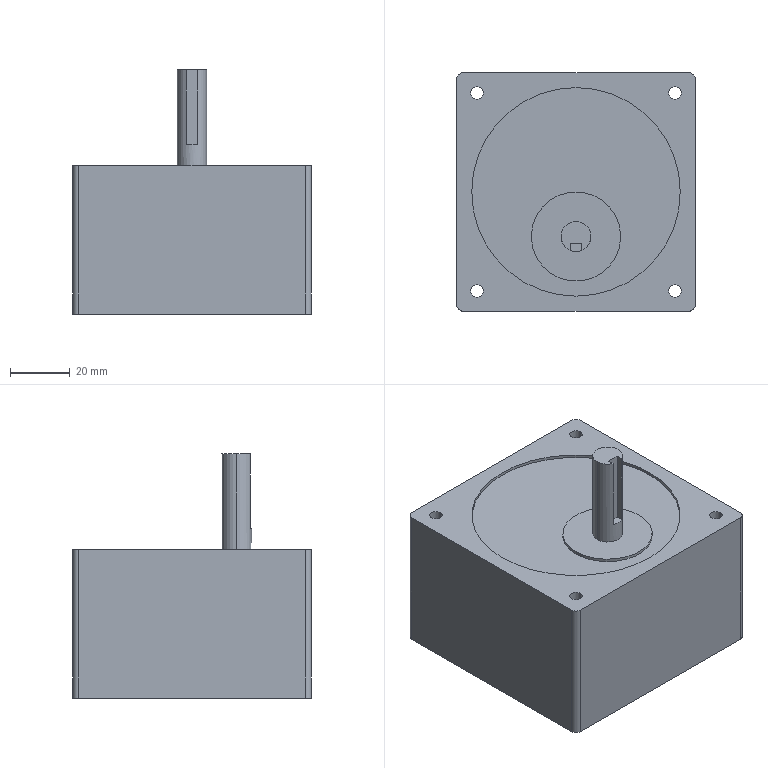Part | SolidWorks | features ICE 5, 3DProfileFeature 1, Extrusion 1, Fillet 1, HoleWzd 1 | 1 solid | 34 faces | box 80 x 80 x 82 mm | volume 314622 mm3 | cylinder 20 | plane 14 | commonest cylinder face diameters 4.2 x8 4 x4 10 x4 30 x2 70 x2
STEP:
#1=CARTESIAN_POINT('',(45.,25.,82.));
#2=VERTEX_POINT('',#1);
#3=CARTESIAN_POINT('',(35.,25.,82.));
#4=VERTEX_POINT('',#3);
#5=CARTESIAN_POINT('',(40.,25.,82.));
#6=DIRECTION('',(0.,0.,1.));
#7=DIRECTION('',(1.,0.,0.));
#8=AXIS2_PLACEMENT_3D('',#5,#6,#7);
#9=CIRCLE('',#8,5.);
#10=EDGE_CURVE('',#2,#4,#9,.T.);
#11=ORIENTED_EDGE('',*,*,#10,.F.);
#12=CARTESIAN_POINT('',(45.,25.,50.));
#13=VERTEX_POINT('',#12);
#14=CARTESIAN_POINT('',(45.,25.,82.));
#15=DIRECTION('',(0.,0.,-1.));
#16=VECTOR('',#15,1000.);
#17=LINE('',#14,#16);
#18=EDGE_CURVE('',#2,#13,#17,.T.);
#19=ORIENTED_EDGE('',*,*,#18,.T.);
#20=CARTESIAN_POINT('',(35.,25.,50.));
#21=VERTEX_POINT('',#20);
#22=CARTESIAN_POINT('',(40.,25.,50.));
#23=DIRECTION('',(0.,0.,1.));
#24=DIRECTION('',(1.,0.,0.));
#25=AXIS2_PLACEMENT_3D('',#22,#23,#24);
#26=CIRCLE('',#25,5.);
#27=EDGE_CURVE('',#13,#21,#26,.T.);
#28=ORIENTED_EDGE('',*,*,#27,.T.);
#29=CARTESIAN_POINT('',(35.,25.,82.));
#30=DIRECTION('',(0.,0.,-1.));
#31=VECTOR('',#30,1000.);
#32=LINE('',#29,#31);
#33=EDGE_CURVE('',#4,#21,#32,.T.);
#34=ORIENTED_EDGE('',*,*,#33,.F.);
#35=EDGE_LOOP('',(#11,#19,#28,#34));
#36=FACE_OUTER_BOUND('',#35,.T.);
#37=CARTESIAN_POINT('',(40.,25.,82.));
#38=DIRECTION('',(0.,0.,-1.));
#39=DIRECTION('',(-1.,0.,0.));
#40=AXIS2_PLACEMENT_3D('',#37,#38,#39);
#41=CYLINDRICAL_SURFACE('',#40,5.);
#42=ADVANCED_FACE('',(#36),#41,.T.);
#43=CARTESIAN_POINT('',(55.,25.,50.));
#44=VERTEX_POINT('',#43);
#45=CARTESIAN_POINT('',(25.,25.,50.));
#46=VERTEX_POINT('',#45);
#47=CARTESIAN_POINT('',(40.,25.,50.));
#48=DIRECTION('',(0.,0.,1.));
#49=DIRECTION('',(1.,0.,0.));
#50=AXIS2_PLACEMENT_3D('',#47,#48,#49);
#51=CIRCLE('',#50,15.);
#52=EDGE_CURVE('',#44,#46,#51,.T.);
#53=ORIENTED_EDGE('',*,*,#52,.F.);
#54=CARTESIAN_POINT('',(55.,25.,49.));
#55=VERTEX_POINT('',#54);
#56=CARTESIAN_POINT('',(55.,25.,50.));
#57=DIRECTION('',(0.,0.,-1.));
#58=VECTOR('',#57,1000.);
#59=LINE('',#56,#58);
#60=EDGE_CURVE('',#44,#55,#59,.T.);
#61=ORIENTED_EDGE('',*,*,#60,.T.);
#62=CARTESIAN_POINT('',(25.,25.,49.));
#63=VERTEX_POINT('',#62);
#64=CARTESIAN_POINT('',(40.,25.,49.));
#65=DIRECTION('',(0.,0.,1.));
#66=DIRECTION('',(1.,0.,0.));
#67=AXIS2_PLACEMENT_3D('',#64,#65,#66);
#68=CIRCLE('',#67,15.);
#69=EDGE_CURVE('',#55,#63,#68,.T.);
#70=ORIENTED_EDGE('',*,*,#69,.T.);
#71=CARTESIAN_POINT('',(25.,25.,50.));
#72=DIRECTION('',(0.,0.,-1.));
#73=VECTOR('',#72,1000.);
#74=LINE('',#71,#73);
#75=EDGE_CURVE('',#46,#63,#74,.T.);
#76=ORIENTED_EDGE('',*,*,#75,.F.);
#77=EDGE_LOOP('',(#53,#61,#70,#76));
#78=FACE_OUTER_BOUND('',#77,.T.);
#79=CARTESIAN_POINT('',(40.,25.,50.));
#80=DIRECTION('',(0.,0.,-1.));
#81=DIRECTION('',(-1.,0.,0.));
#82=AXIS2_PLACEMENT_3D('',#79,#80,#81);
#83=CYLINDRICAL_SURFACE('',#82,15.);
#84=ADVANCED_FACE('',(#78),#83,.T.);
#85=CARTESIAN_POINT('',(45.,40.,20.));
#86=VERTEX_POINT('',#85);
#87=CARTESIAN_POINT('',(35.,40.,20.));
#88=VERTEX_POINT('',#87);
#89=CARTESIAN_POINT('',(40.,40.,20.));
#90=DIRECTION('',(0.,0.,-1.));
#91=DIRECTION('',(-1.,0.,0.));
#92=AXIS2_PLACEMENT_3D('',#89,#90,#91);
#93=CIRCLE('',#92,5.);
#94=EDGE_CURVE('',#86,#88,#93,.T.);
#95=ORIENTED_EDGE('',*,*,#94,.F.);
#96=CARTESIAN_POINT('',(45.,40.,0.));
#97=VERTEX_POINT('',#96);
#98=CARTESIAN_POINT('',(45.,40.,20.));
#99=DIRECTION('',(0.,0.,-1.));
#100=VECTOR('',#99,1000.);
#101=LINE('',#98,#100);
#102=EDGE_CURVE('',#86,#97,#101,.T.);
#103=ORIENTED_EDGE('',*,*,#102,.T.);
#104=CARTESIAN_POINT('',(35.,40.,0.));
#105=VERTEX_POINT('',#104);
#106=CARTESIAN_POINT('',(40.,40.,0.));
#107=DIRECTION('',(0.,0.,-1.));
#108=DIRECTION('',(-1.,0.,0.));
#109=AXIS2_PLACEMENT_3D('',#106,#107,#108);
#110=CIRCLE('',#109,5.);
#111=EDGE_CURVE('',#97,#105,#110,.T.);
#112=ORIENTED_EDGE('',*,*,#111,.T.);
#113=CARTESIAN_POINT('',(35.,40.,20.));
#114=DIRECTION('',(0.,0.,-1.));
#115=VECTOR('',#114,1000.);
#116=LINE('',#113,#115);
#117=EDGE_CURVE('',#88,#105,#116,.T.);
#118=ORIENTED_EDGE('',*,*,#117,.F.);
#119=EDGE_LOOP('',(#95,#103,#112,#118));
#120=FACE_OUTER_BOUND('',#119,.T.);
#121=CARTESIAN_POINT('',(40.,40.,20.));
#122=DIRECTION('',(0.,0.,-1.));
#123=DIRECTION('',(-1.,0.,0.));
#124=AXIS2_PLACEMENT_3D('',#121,#122,#123);
#125=CYLINDRICAL_SURFACE('',#124,5.);
#126=ADVANCED_FACE('',(#120),#125,.F.);
#127=CARTESIAN_POINT('',(75.334,73.234,50.));
#128=VERTEX_POINT('',#127);
#129=CARTESIAN_POINT('',(71.134,73.234,50.));
#130=VERTEX_POINT('',#129);
#131=CARTESIAN_POINT('',(73.234,73.234,50.));
#132=DIRECTION('',(0.,0.,-1.));
#133=DIRECTION('',(-1.,0.,0.));
#134=AXIS2_PLACEMENT_3D('',#131,#132,#133);
#135=CIRCLE('',#134,2.1);
#136=EDGE_CURVE('',#128,#130,#135,.T.);
#137=ORIENTED_EDGE('',*,*,#136,.F.);
#138=CARTESIAN_POINT('',(75.334,73.234,0.));
#139=VERTEX_POINT('',#138);
#140=CARTESIAN_POINT('',(75.334,73.234,0.));
#141=DIRECTION('',(0.,0.,-1.));
#142=VECTOR('',#141,1000.);
#143=LINE('',#140,#142);
#144=EDGE_CURVE('',#128,#139,#143,.T.);
#145=ORIENTED_EDGE('',*,*,#144,.T.);
#146=CARTESIAN_POINT('',(71.134,73.234,0.));
#147=VERTEX_POINT('',#146);
#148=CARTESIAN_POINT('',(73.234,73.234,0.));
#149=DIRECTION('',(0.,0.,-1.));
#150=DIRECTION('',(-1.,0.,0.));
#151=AXIS2_PLACEMENT_3D('',#148,#149,#150);
#152=CIRCLE('',#151,2.1);
#153=EDGE_CURVE('',#139,#147,#152,.T.);
#154=ORIENTED_EDGE('',*,*,#153,.T.);
#155=CARTESIAN_POINT('',(71.134,73.234,0.));
#156=DIRECTION('',(0.,0.,-1.));
#157=VECTOR('',#156,1000.);
#158=LINE('',#155,#157);
#159=EDGE_CURVE('',#130,#147,#158,.T.);
#160=ORIENTED_EDGE('',*,*,#159,.F.);
#161=EDGE_LOOP('',(#137,#145,#154,#160));
#162=FACE_OUTER_BOUND('',#161,.T.);
#163=CARTESIAN_POINT('',(73.234,73.234,0.));
#164=DIRECTION('',(0.,0.,-1.));
#165=DIRECTION('',(-1.,0.,0.));
#166=AXIS2_PLACEMENT_3D('',#163,#164,#165);
#167=CYLINDRICAL_SURFACE('',#166,2.1);
#168=ADVANCED_FACE('',(#162),#167,.F.);
#169=CARTESIAN_POINT('',(8.866,73.234,50.));
#170=VERTEX_POINT('',#169);
#171=CARTESIAN_POINT('',(4.666,73.234,50.));
#172=VERTEX_POINT('',#171);
#173=CARTESIAN_POINT('',(6.766,73.234,50.));
#174=DIRECTION('',(0.,0.,-1.));
#175=DIRECTION('',(-1.,0.,0.));
#176=AXIS2_PLACEMENT_3D('',#173,#174,#175);
#177=CIRCLE('',#176,2.1);
#178=EDGE_CURVE('',#170,#172,#177,.T.);
#179=ORIENTED_EDGE('',*,*,#178,.F.);
#180=CARTESIAN_POINT('',(8.866,73.234,0.));
#181=VERTEX_POINT('',#180);
#182=CARTESIAN_POINT('',(8.866,73.234,0.));
#183=DIRECTION('',(0.,0.,-1.));
#184=VECTOR('',#183,1000.);
#185=LINE('',#182,#184);
#186=EDGE_CURVE('',#170,#181,#185,.T.);
#187=ORIENTED_EDGE('',*,*,#186,.T.);
#188=CARTESIAN_POINT('',(4.666,73.234,0.));
#189=VERTEX_POINT('',#188);
#190=CARTESIAN_POINT('',(6.766,73.234,0.));
#191=DIRECTION('',(0.,0.,-1.));
#192=DIRECTION('',(-1.,0.,0.));
#193=AXIS2_PLACEMENT_3D('',#190,#191,#192);
#194=CIRCLE('',#193,2.1);
#195=EDGE_CURVE('',#181,#189,#194,.T.);
#196=ORIENTED_EDGE('',*,*,#195,.T.);
#197=CARTESIAN_POINT('',(4.666,73.234,0.));
#198=DIRECTION('',(0.,0.,-1.));
#199=VECTOR('',#198,1000.);
#200=LINE('',#197,#199);
#201=EDGE_CURVE('',#172,#189,#200,.T.);
#202=ORIENTED_EDGE('',*,*,#201,.F.);
#203=EDGE_LOOP('',(#179,#187,#196,#202));
#204=FACE_OUTER_BOUND('',#203,.T.);
#205=CARTESIAN_POINT('',(6.766,73.234,0.));
#206=DIRECTION('',(0.,0.,-1.));
#207=DIRECTION('',(-1.,0.,0.));
#208=AXIS2_PLACEMENT_3D('',#205,#206,#207);
#209=CYLINDRICAL_SURFACE('',#208,2.1);
#210=ADVANCED_FACE('',(#204),#209,.F.);
#211=CARTESIAN_POINT('',(8.866,6.766,50.));
#212=VERTEX_POINT('',#211);
#213=CARTESIAN_POINT('',(4.666,6.766,50.));
#214=VERTEX_POINT('',#213);
#215=CARTESIAN_POINT('',(6.766,6.766,50.));
#216=DIRECTION('',(0.,0.,-1.));
#217=DIRECTION('',(-1.,0.,0.));
#218=AXIS2_PLACEMENT_3D('',#215,#216,#217);
#219=CIRCLE('',#218,2.1);
#220=EDGE_CURVE('',#212,#214,#219,.T.);
#221=ORIENTED_EDGE('',*,*,#220,.F.);
#222=CARTESIAN_POINT('',(8.866,6.766,0.));
#223=VERTEX_POINT('',#222);
#224=CARTESIAN_POINT('',(8.866,6.766,0.));
#225=DIRECTION('',(0.,0.,-1.));
#226=VECTOR('',#225,1000.);
#227=LINE('',#224,#226);
#228=EDGE_CURVE('',#212,#223,#227,.T.);
#229=ORIENTED_EDGE('',*,*,#228,.T.);
#230=CARTESIAN_POINT('',(4.666,6.766,0.));
#231=VERTEX_POINT('',#230);
#232=CARTESIAN_POINT('',(6.766,6.766,0.));
#233=DIRECTION('',(0.,0.,-1.));
#234=DIRECTION('',(-1.,0.,0.));
#235=AXIS2_PLACEMENT_3D('',#232,#233,#234);
#236=CIRCLE('',#235,2.1);
#237=EDGE_CURVE('',#223,#231,#236,.T.);
#238=ORIENTED_EDGE('',*,*,#237,.T.);
#239=CARTESIAN_POINT('',(4.666,6.766,0.));
#240=DIRECTION('',(0.,0.,-1.));
#241=VECTOR('',#240,1000.);
#242=LINE('',#239,#241);
#243=EDGE_CURVE('',#214,#231,#242,.T.);
#244=ORIENTED_EDGE('',*,*,#243,.F.);
#245=EDGE_LOOP('',(#221,#229,#238,#244));
#246=FACE_OUTER_BOUND('',#245,.T.);
#247=CARTESIAN_POINT('',(6.766,6.766,0.));
#248=DIRECTION('',(0.,0.,-1.));
#249=DIRECTION('',(-1.,0.,0.));
#250=AXIS2_PLACEMENT_3D('',#247,#248,#249);
#251=CYLINDRICAL_SURFACE('',#250,2.1);
#252=ADVANCED_FACE('',(#246),#251,.F.);
#253=CARTESIAN_POINT('',(75.334,6.766,50.));
#254=VERTEX_POINT('',#253);
#255=CARTESIAN_POINT('',(71.134,6.766,50.));
#256=VERTEX_POINT('',#255);
#257=CARTESIAN_POINT('',(73.234,6.766,50.));
#258=DIRECTION('',(0.,0.,-1.));
#259=DIRECTION('',(-1.,0.,0.));
#260=AXIS2_PLACEMENT_3D('',#257,#258,#259);
#261=CIRCLE('',#260,2.1);
#262=EDGE_CURVE('',#254,#256,#261,.T.);
#263=ORIENTED_EDGE('',*,*,#262,.F.);
#264=CARTESIAN_POINT('',(75.334,6.766,0.));
#265=VERTEX_POINT('',#264);
#266=CARTESIAN_POINT('',(75.334,6.766,0.));
#267=DIRECTION('',(0.,0.,-1.));
#268=VECTOR('',#267,1000.);
#269=LINE('',#266,#268);
#270=EDGE_CURVE('',#254,#265,#269,.T.);
#271=ORIENTED_EDGE('',*,*,#270,.T.);
#272=CARTESIAN_POINT('',(71.134,6.766,0.));
#273=VERTEX_POINT('',#272);
#274=CARTESIAN_POINT('',(73.234,6.766,0.));
#275=DIRECTION('',(0.,0.,-1.));
#276=DIRECTION('',(-1.,0.,0.));
#277=AXIS2_PLACEMENT_3D('',#274,#275,#276);
#278=CIRCLE('',#277,2.1);
#279=EDGE_CURVE('',#265,#273,#278,.T.);
#280=ORIENTED_EDGE('',*,*,#279,.T.);
#281=CARTESIAN_POINT('',(71.134,6.766,0.));
#282=DIRECTION('',(0.,0.,-1.));
#283=VECTOR('',#282,1000.);
#284=LINE('',#281,#283);
#285=EDGE_CURVE('',#256,#273,#284,.T.);
#286=ORIENTED_EDGE('',*,*,#285,.F.);
#287=EDGE_LOOP('',(#263,#271,#280,#286));
#288=FACE_OUTER_BOUND('',#287,.T.);
#289=CARTESIAN_POINT('',(73.234,6.766,0.));
#290=DIRECTION('',(0.,0.,-1.));
#291=DIRECTION('',(-1.,0.,0.));
#292=AXIS2_PLACEMENT_3D('',#289,#290,#291);
#293=CYLINDRICAL_SURFACE('',#292,2.1);
#294=ADVANCED_FACE('',(#288),#293,.F.);
#295=CARTESIAN_POINT('',(5.,40.,49.));
#296=VERTEX_POINT('',#295);
#297=CARTESIAN_POINT('',(75.,40.,49.));
#298=VERTEX_POINT('',#297);
#299=CARTESIAN_POINT('',(40.,40.,49.));
#300=DIRECTION('',(0.,0.,1.));
#301=DIRECTION('',(1.,0.,0.));
#302=AXIS2_PLACEMENT_3D('',#299,#300,#301);
#303=CIRCLE('',#302,35.);
#304=EDGE_CURVE('',#296,#298,#303,.T.);
#305=ORIENTED_EDGE('',*,*,#304,.F.);
#306=CARTESIAN_POINT('',(5.,40.,50.));
#307=VERTEX_POINT('',#306);
#308=CARTESIAN_POINT('',(5.,40.,49.));
#309=DIRECTION('',(0.,0.,1.));
#310=VECTOR('',#309,1000.);
#311=LINE('',#308,#310);
#312=EDGE_CURVE('',#296,#307,#311,.T.);
#313=ORIENTED_EDGE('',*,*,#312,.T.);
#314=CARTESIAN_POINT('',(75.,40.,50.));
#315=VERTEX_POINT('',#314);
#316=CARTESIAN_POINT('',(40.,40.,50.));
#317=DIRECTION('',(0.,0.,1.));
#318=DIRECTION('',(1.,0.,0.));
#319=AXIS2_PLACEMENT_3D('',#316,#317,#318);
#320=CIRCLE('',#319,35.);
#321=EDGE_CURVE('',#307,#315,#320,.T.);
#322=ORIENTED_EDGE('',*,*,#321,.T.);
#323=CARTESIAN_POINT('',(75.,40.,49.));
#324=DIRECTION('',(0.,0.,1.));
#325=VECTOR('',#324,1000.);
#326=LINE('',#323,#325);
#327=EDGE_CURVE('',#298,#315,#326,.T.);
#328=ORIENTED_EDGE('',*,*,#327,.F.);
#329=EDGE_LOOP('',(#305,#313,#322,#328));
#330=FACE_OUTER_BOUND('',#329,.T.);
#331=CARTESIAN_POINT('',(40.,40.,49.));
#332=DIRECTION('',(0.,0.,1.));
#333=DIRECTION('',(1.,0.,0.));
#334=AXIS2_PLACEMENT_3D('',#331,#332,#333);
#335=CYLINDRICAL_SURFACE('',#334,35.);
#336=ADVANCED_FACE('',(#330),#335,.F.);
#337=CARTESIAN_POINT('',(40.,25.,50.));
#338=DIRECTION('',(0.,0.,1.));
#339=DIRECTION('',(1.,0.,0.));
#340=AXIS2_PLACEMENT_3D('',#337,#338,#339);
#341=CIRCLE('',#340,15.);
#342=EDGE_CURVE('',#46,#44,#341,.T.);
#343=ORIENTED_EDGE('',*,*,#342,.T.);
#344=ORIENTED_EDGE('',*,*,#52,.T.);
#345=EDGE_LOOP('',(#343,#344));
#346=FACE_OUTER_BOUND('',#345,.T.);
#347=CARTESIAN_POINT('',(40.,25.,50.));
#348=DIRECTION('',(0.,0.,1.));
#349=DIRECTION('',(1.,0.,0.));
#350=AXIS2_PLACEMENT_3D('',#347,#348,#349);
#351=CIRCLE('',#350,5.);
#352=EDGE_CURVE('',#21,#13,#351,.T.);
#353=ORIENTED_EDGE('',*,*,#352,.F.);
#354=ORIENTED_EDGE('',*,*,#27,.F.);
#355=EDGE_LOOP('',(#353,#354));
#356=FACE_BOUND('',#355,.T.);
#357=CARTESIAN_POINT('',(40.,25.,50.));
#358=DIRECTION('',(0.,0.,1.));
#359=DIRECTION('',(1.,0.,0.));
#360=AXIS2_PLACEMENT_3D('',#357,#358,#359);
#361=PLANE('',#360);
#362=ADVANCED_FACE('',(#346,#356),#361,.T.);
#363=CARTESIAN_POINT('',(40.,40.,49.));
#364=DIRECTION('',(0.,0.,1.));
#365=DIRECTION('',(1.,0.,0.));
#366=AXIS2_PLACEMENT_3D('',#363,#364,#365);
#367=CIRCLE('',#366,35.);
#368=EDGE_CURVE('',#298,#296,#367,.T.);
#369=ORIENTED_EDGE('',*,*,#368,.T.);
#370=ORIENTED_EDGE('',*,*,#304,.T.);
#371=EDGE_LOOP('',(#369,#370));
#372=FACE_OUTER_BOUND('',#371,.T.);
#373=CARTESIAN_POINT('',(40.,25.,49.));
#374=DIRECTION('',(0.,0.,1.));
#375=DIRECTION('',(1.,0.,0.));
#376=AXIS2_PLACEMENT_3D('',#373,#374,#375);
#377=CIRCLE('',#376,15.);
#378=EDGE_CURVE('',#63,#55,#377,.T.);
#379=ORIENTED_EDGE('',*,*,#378,.F.);
#380=ORIENTED_EDGE('',*,*,#69,.F.);
#381=EDGE_LOOP('',(#379,#380));
#382=FACE_BOUND('',#381,.T.);
#383=CARTESIAN_POINT('',(40.,40.,49.));
#384=DIRECTION('',(0.,0.,1.));
#385=DIRECTION('',(1.,0.,0.));
#386=AXIS2_PLACEMENT_3D('',#383,#384,#385);
#387=PLANE('',#386);
#388=ADVANCED_FACE('',(#372,#382),#387,.T.);
#389=CARTESIAN_POINT('',(0.,78.,50.));
#390=VERTEX_POINT('',#389);
#391=CARTESIAN_POINT('',(0.,2.,50.));
#392=VERTEX_POINT('',#391);
#393=CARTESIAN_POINT('',(0.,0.,50.));
#394=DIRECTION('',(0.,-1.,0.));
#395=VECTOR('',#394,1000.);
#396=LINE('',#393,#395);
#397=EDGE_CURVE('',#390,#392,#396,.T.);
#398=ORIENTED_EDGE('',*,*,#397,.F.);
#399=CARTESIAN_POINT('',(0.,78.,0.));
#400=VERTEX_POINT('',#399);
#401=CARTESIAN_POINT('',(0.,78.,50.));
#402=DIRECTION('',(0.,0.,-1.));
#403=VECTOR('',#402,1000.);
#404=LINE('',#401,#403);
#405=EDGE_CURVE('',#390,#400,#404,.T.);
#406=ORIENTED_EDGE('',*,*,#405,.T.);
#407=CARTESIAN_POINT('',(0.,2.,0.));
#408=VERTEX_POINT('',#407);
#409=CARTESIAN_POINT('',(0.,0.,0.));
#410=DIRECTION('',(0.,-1.,0.));
#411=VECTOR('',#410,1000.);
#412=LINE('',#409,#411);
#413=EDGE_CURVE('',#400,#408,#412,.T.);
#414=ORIENTED_EDGE('',*,*,#413,.T.);
#415=CARTESIAN_POINT('',(0.,2.,50.));
#416=DIRECTION('',(0.,0.,1.));
#417=VECTOR('',#416,1000.);
#418=LINE('',#415,#417);
#419=EDGE_CURVE('',#408,#392,#418,.T.);
#420=ORIENTED_EDGE('',*,*,#419,.T.);
#421=EDGE_LOOP('',(#398,#406,#414,#420));
#422=FACE_OUTER_BOUND('',#421,.T.);
#423=CARTESIAN_POINT('',(0.,0.,50.));
#424=DIRECTION('',(1.,0.,0.));
#425=DIRECTION('',(0.,0.,-1.));
#426=AXIS2_PLACEMENT_3D('',#423,#424,#425);
#427=PLANE('',#426);
#428=ADVANCED_FACE('',(#422),#427,.F.);
#429=CARTESIAN_POINT('',(2.,0.,0.));
#430=VERTEX_POINT('',#429);
#431=CARTESIAN_POINT('',(78.,0.,0.));
#432=VERTEX_POINT('',#431);
#433=CARTESIAN_POINT('',(0.,0.,0.));
#434=DIRECTION('',(1.,0.,0.));
#435=VECTOR('',#434,1000.);
#436=LINE('',#433,#435);
#437=EDGE_CURVE('',#430,#432,#436,.T.);
#438=ORIENTED_EDGE('',*,*,#437,.T.);
#439=CARTESIAN_POINT('',(78.,0.,50.));
#440=VERTEX_POINT('',#439);
#441=CARTESIAN_POINT('',(78.,0.,50.));
#442=DIRECTION('',(0.,0.,1.));
#443=VECTOR('',#442,1000.);
#444=LINE('',#441,#443);
#445=EDGE_CURVE('',#432,#440,#444,.T.);
#446=ORIENTED_EDGE('',*,*,#445,.T.);
#447=CARTESIAN_POINT('',(2.,0.,50.));
#448=VERTEX_POINT('',#447);
#449=CARTESIAN_POINT('',(0.,0.,50.));
#450=DIRECTION('',(1.,0.,0.));
#451=VECTOR('',#450,1000.);
#452=LINE('',#449,#451);
#453=EDGE_CURVE('',#448,#440,#452,.T.);
#454=ORIENTED_EDGE('',*,*,#453,.F.);
#455=CARTESIAN_POINT('',(2.,0.,50.));
#456=DIRECTION('',(0.,0.,-1.));
#457=VECTOR('',#456,1000.);
#458=LINE('',#455,#457);
#459=EDGE_CURVE('',#448,#430,#458,.T.);
#460=ORIENTED_EDGE('',*,*,#459,.T.);
#461=EDGE_LOOP('',(#438,#446,#454,#460));
#462=FACE_OUTER_BOUND('',#461,.T.);
#463=CARTESIAN_POINT('',(0.,0.,50.));
#464=DIRECTION('',(0.,1.,0.));
#465=DIRECTION('',(0.,0.,1.));
#466=AXIS2_PLACEMENT_3D('',#463,#464,#465);
#467=PLANE('',#466);
#468=ADVANCED_FACE('',(#462),#467,.F.);
#469=CARTESIAN_POINT('',(80.,2.,50.));
#470=VERTEX_POINT('',#469);
#471=CARTESIAN_POINT('',(80.,78.,50.));
#472=VERTEX_POINT('',#471);
#473=CARTESIAN_POINT('',(80.,0.,50.));
#474=DIRECTION('',(0.,1.,0.));
#475=VECTOR('',#474,1000.);
#476=LINE('',#473,#475);
#477=EDGE_CURVE('',#470,#472,#476,.T.);
#478=ORIENTED_EDGE('',*,*,#477,.F.);
#479=CARTESIAN_POINT('',(80.,2.,0.));
#480=VERTEX_POINT('',#479);
#481=CARTESIAN_POINT('',(80.,2.,50.));
#482=DIRECTION('',(0.,0.,-1.));
#483=VECTOR('',#482,1000.);
#484=LINE('',#481,#483);
#485=EDGE_CURVE('',#470,#480,#484,.T.);
#486=ORIENTED_EDGE('',*,*,#485,.T.);
#487=CARTESIAN_POINT('',(80.,78.,0.));
#488=VERTEX_POINT('',#487);
#489=CARTESIAN_POINT('',(80.,0.,0.));
#490=DIRECTION('',(0.,1.,0.));
#491=VECTOR('',#490,1000.);
#492=LINE('',#489,#491);
#493=EDGE_CURVE('',#480,#488,#492,.T.);
#494=ORIENTED_EDGE('',*,*,#493,.T.);
#495=CARTESIAN_POINT('',(80.,78.,50.));
#496=DIRECTION('',(0.,0.,1.));
#497=VECTOR('',#496,1000.);
#498=LINE('',#495,#497);
#499=EDGE_CURVE('',#488,#472,#498,.T.);
#500=ORIENTED_EDGE('',*,*,#499,.T.);
#501=EDGE_LOOP('',(#478,#486,#494,#500));
#502=FACE_OUTER_BOUND('',#501,.T.);
#503=CARTESIAN_POINT('',(80.,0.,50.));
#504=DIRECTION('',(-1.,0.,0.));
#505=DIRECTION('',(0.,-1.,0.));
#506=AXIS2_PLACEMENT_3D('',#503,#504,#505);
#507=PLANE('',#506);
#508=ADVANCED_FACE('',(#502),#507,.F.);
#509=CARTESIAN_POINT('',(78.,80.,50.));
#510=VERTEX_POINT('',#509);
#511=CARTESIAN_POINT('',(2.,80.,50.));
#512=VERTEX_POINT('',#511);
#513=CARTESIAN_POINT('',(0.,80.,50.));
#514=DIRECTION('',(-1.,0.,0.));
#515=VECTOR('',#514,1000.);
#516=LINE('',#513,#515);
#517=EDGE_CURVE('',#510,#512,#516,.T.);
#518=ORIENTED_EDGE('',*,*,#517,.F.);
#519=CARTESIAN_POINT('',(78.,80.,0.));
#520=VERTEX_POINT('',#519);
#521=CARTESIAN_POINT('',(78.,80.,50.));
#522=DIRECTION('',(0.,0.,-1.));
#523=VECTOR('',#522,1000.);
#524=LINE('',#521,#523);
#525=EDGE_CURVE('',#510,#520,#524,.T.);
#526=ORIENTED_EDGE('',*,*,#525,.T.);
#527=CARTESIAN_POINT('',(2.,80.,0.));
#528=VERTEX_POINT('',#527);
#529=CARTESIAN_POINT('',(0.,80.,0.));
#530=DIRECTION('',(-1.,0.,0.));
#531=VECTOR('',#530,1000.);
#532=LINE('',#529,#531);
#533=EDGE_CURVE('',#520,#528,#532,.T.);
#534=ORIENTED_EDGE('',*,*,#533,.T.);
#535=CARTESIAN_POINT('',(2.,80.,50.));
#536=DIRECTION('',(0.,0.,1.));
#537=VECTOR('',#536,1000.);
#538=LINE('',#535,#537);
#539=EDGE_CURVE('',#528,#512,#538,.T.);
#540=ORIENTED_EDGE('',*,*,#539,.T.);
#541=EDGE_LOOP('',(#518,#526,#534,#540));
#542=FACE_OUTER_BOUND('',#541,.T.);
#543=CARTESIAN_POINT('',(0.,80.,50.));
#544=DIRECTION('',(0.,-1.,0.));
#545=DIRECTION('',(1.,0.,0.));
#546=AXIS2_PLACEMENT_3D('',#543,#544,#545);
#547=PLANE('',#546);
#548=ADVANCED_FACE('',(#542),#547,.F.);
#549=CARTESIAN_POINT('',(73.234,73.234,50.));
#550=DIRECTION('',(0.,0.,-1.));
#551=DIRECTION('',(-1.,0.,0.));
#552=AXIS2_PLACEMENT_3D('',#549,#550,#551);
#553=CIRCLE('',#552,2.1);
#554=EDGE_CURVE('',#130,#128,#553,.T.);
#555=ORIENTED_EDGE('',*,*,#554,.T.);
#556=ORIENTED_EDGE('',*,*,#136,.T.);
#557=EDGE_LOOP('',(#555,#556));
#558=FACE_BOUND('',#557,.T.);
#559=CARTESIAN_POINT('',(6.766,73.234,50.));
#560=DIRECTION('',(0.,0.,-1.));
#561=DIRECTION('',(-1.,0.,0.));
#562=AXIS2_PLACEMENT_3D('',#559,#560,#561);
#563=CIRCLE('',#562,2.1);
#564=EDGE_CURVE('',#172,#170,#563,.T.);
#565=ORIENTED_EDGE('',*,*,#564,.T.);
#566=ORIENTED_EDGE('',*,*,#178,.T.);
#567=EDGE_LOOP('',(#565,#566));
#568=FACE_BOUND('',#567,.T.);
#569=CARTESIAN_POINT('',(6.766,6.766,50.));
#570=DIRECTION('',(0.,0.,-1.));
#571=DIRECTION('',(-1.,0.,0.));
#572=AXIS2_PLACEMENT_3D('',#569,#570,#571);
#573=CIRCLE('',#572,2.1);
#574=EDGE_CURVE('',#214,#212,#573,.T.);
#575=ORIENTED_EDGE('',*,*,#574,.T.);
#576=ORIENTED_EDGE('',*,*,#220,.T.);
#577=EDGE_LOOP('',(#575,#576));
#578=FACE_BOUND('',#577,.T.);
#579=CARTESIAN_POINT('',(73.234,6.766,50.));
#580=DIRECTION('',(0.,0.,-1.));
#581=DIRECTION('',(-1.,0.,0.));
#582=AXIS2_PLACEMENT_3D('',#579,#580,#581);
#583=CIRCLE('',#582,2.1);
#584=EDGE_CURVE('',#256,#254,#583,.T.);
#585=ORIENTED_EDGE('',*,*,#584,.T.);
#586=ORIENTED_EDGE('',*,*,#262,.T.);
#587=EDGE_LOOP('',(#585,#586));
#588=FACE_BOUND('',#587,.T.);
#589=CARTESIAN_POINT('',(40.,40.,50.));
#590=DIRECTION('',(0.,0.,1.));
#591=DIRECTION('',(1.,0.,0.));
#592=AXIS2_PLACEMENT_3D('',#589,#590,#591);
#593=CIRCLE('',#592,35.);
#594=EDGE_CURVE('',#315,#307,#593,.T.);
#595=ORIENTED_EDGE('',*,*,#594,.F.);
#596=ORIENTED_EDGE('',*,*,#321,.F.);
#597=EDGE_LOOP('',(#595,#596));
#598=FACE_BOUND('',#597,.T.);
#599=ORIENTED_EDGE('',*,*,#453,.T.);
#600=CARTESIAN_POINT('',(78.,2.,50.));
#601=DIRECTION('',(0.,0.,1.));
#602=DIRECTION('',(-1.,0.,0.));
#603=AXIS2_PLACEMENT_3D('',#600,#601,#602);
#604=CIRCLE('',#603,2.);
#605=EDGE_CURVE('',#440,#470,#604,.T.);
#606=ORIENTED_EDGE('',*,*,#605,.T.);
#607=ORIENTED_EDGE('',*,*,#477,.T.);
#608=CARTESIAN_POINT('',(78.,78.,50.));
#609=DIRECTION('',(0.,0.,1.));
#610=DIRECTION('',(-1.,0.,0.));
#611=AXIS2_PLACEMENT_3D('',#608,#609,#610);
#612=CIRCLE('',#611,2.);
#613=EDGE_CURVE('',#472,#510,#612,.T.);
#614=ORIENTED_EDGE('',*,*,#613,.T.);
#615=ORIENTED_EDGE('',*,*,#517,.T.);
#616=CARTESIAN_POINT('',(2.,78.,50.));
#617=DIRECTION('',(0.,0.,1.));
#618=DIRECTION('',(-1.,0.,0.));
#619=AXIS2_PLACEMENT_3D('',#616,#617,#618);
#620=CIRCLE('',#619,2.);
#621=EDGE_CURVE('',#512,#390,#620,.T.);
#622=ORIENTED_EDGE('',*,*,#621,.T.);
#623=ORIENTED_EDGE('',*,*,#397,.T.);
#624=CARTESIAN_POINT('',(2.,2.,50.));
#625=DIRECTION('',(0.,0.,1.));
#626=DIRECTION('',(-1.,0.,0.));
#627=AXIS2_PLACEMENT_3D('',#624,#625,#626);
#628=CIRCLE('',#627,2.);
#629=EDGE_CURVE('',#392,#448,#628,.T.);
#630=ORIENTED_EDGE('',*,*,#629,.T.);
#631=EDGE_LOOP('',(#599,#606,#607,#614,#615,#622,#623,#630));
#632=FACE_OUTER_BOUND('',#631,.T.);
#633=CARTESIAN_POINT('',(0.,0.,50.));
#634=DIRECTION('',(0.,0.,-1.));
#635=DIRECTION('',(-1.,0.,0.));
#636=AXIS2_PLACEMENT_3D('',#633,#634,#635);
#637=PLANE('',#636);
#638=ADVANCED_FACE('',(#558,#568,#578,#588,#598,#632),#637,.F.);
#639=CARTESIAN_POINT('',(40.,40.,0.));
#640=DIRECTION('',(0.,0.,-1.));
#641=DIRECTION('',(-1.,0.,0.));
#642=AXIS2_PLACEMENT_3D('',#639,#640,#641);
#643=CIRCLE('',#642,5.);
#644=EDGE_CURVE('',#105,#97,#643,.T.);
#645=ORIENTED_EDGE('',*,*,#644,.F.);
#646=ORIENTED_EDGE('',*,*,#111,.F.);
#647=EDGE_LOOP('',(#645,#646));
#648=FACE_BOUND('',#647,.T.);
#649=CARTESIAN_POINT('',(73.234,73.234,0.));
#650=DIRECTION('',(0.,0.,-1.));
#651=DIRECTION('',(-1.,0.,0.));
#652=AXIS2_PLACEMENT_3D('',#649,#650,#651);
#653=CIRCLE('',#652,2.1);
#654=EDGE_CURVE('',#147,#139,#653,.T.);
#655=ORIENTED_EDGE('',*,*,#654,.F.);
#656=ORIENTED_EDGE('',*,*,#153,.F.);
#657=EDGE_LOOP('',(#655,#656));
#658=FACE_BOUND('',#657,.T.);
#659=CARTESIAN_POINT('',(6.766,73.234,0.));
#660=DIRECTION('',(0.,0.,-1.));
#661=DIRECTION('',(-1.,0.,0.));
#662=AXIS2_PLACEMENT_3D('',#659,#660,#661);
#663=CIRCLE('',#662,2.1);
#664=EDGE_CURVE('',#189,#181,#663,.T.);
#665=ORIENTED_EDGE('',*,*,#664,.F.);
#666=ORIENTED_EDGE('',*,*,#195,.F.);
#667=EDGE_LOOP('',(#665,#666));
#668=FACE_BOUND('',#667,.T.);
#669=CARTESIAN_POINT('',(6.766,6.766,0.));
#670=DIRECTION('',(0.,0.,-1.));
#671=DIRECTION('',(-1.,0.,0.));
#672=AXIS2_PLACEMENT_3D('',#669,#670,#671);
#673=CIRCLE('',#672,2.1);
#674=EDGE_CURVE('',#231,#223,#673,.T.);
#675=ORIENTED_EDGE('',*,*,#674,.F.);
#676=ORIENTED_EDGE('',*,*,#237,.F.);
#677=EDGE_LOOP('',(#675,#676));
#678=FACE_BOUND('',#677,.T.);
#679=CARTESIAN_POINT('',(73.234,6.766,0.));
#680=DIRECTION('',(0.,0.,-1.));
#681=DIRECTION('',(-1.,0.,0.));
#682=AXIS2_PLACEMENT_3D('',#679,#680,#681);
#683=CIRCLE('',#682,2.1);
#684=EDGE_CURVE('',#273,#265,#683,.T.);
#685=ORIENTED_EDGE('',*,*,#684,.F.);
#686=ORIENTED_EDGE('',*,*,#279,.F.);
#687=EDGE_LOOP('',(#685,#686));
#688=FACE_BOUND('',#687,.T.);
#689=ORIENTED_EDGE('',*,*,#493,.F.);
#690=CARTESIAN_POINT('',(78.,2.,0.));
#691=DIRECTION('',(0.,0.,-1.));
#692=DIRECTION('',(-1.,0.,0.));
#693=AXIS2_PLACEMENT_3D('',#690,#691,#692);
#694=CIRCLE('',#693,2.);
#695=EDGE_CURVE('',#480,#432,#694,.T.);
#696=ORIENTED_EDGE('',*,*,#695,.T.);
#697=ORIENTED_EDGE('',*,*,#437,.F.);
#698=CARTESIAN_POINT('',(2.,2.,0.));
#699=DIRECTION('',(0.,0.,-1.));
#700=DIRECTION('',(-1.,0.,0.));
#701=AXIS2_PLACEMENT_3D('',#698,#699,#700);
#702=CIRCLE('',#701,2.);
#703=EDGE_CURVE('',#430,#408,#702,.T.);
#704=ORIENTED_EDGE('',*,*,#703,.T.);
#705=ORIENTED_EDGE('',*,*,#413,.F.);
#706=CARTESIAN_POINT('',(2.,78.,0.));
#707=DIRECTION('',(0.,0.,-1.));
#708=DIRECTION('',(-1.,0.,0.));
#709=AXIS2_PLACEMENT_3D('',#706,#707,#708);
#710=CIRCLE('',#709,2.);
#711=EDGE_CURVE('',#400,#528,#710,.T.);
#712=ORIENTED_EDGE('',*,*,#711,.T.);
#713=ORIENTED_EDGE('',*,*,#533,.F.);
#714=CARTESIAN_POINT('',(78.,78.,0.));
#715=DIRECTION('',(0.,0.,-1.));
#716=DIRECTION('',(-1.,0.,0.));
#717=AXIS2_PLACEMENT_3D('',#714,#715,#716);
#718=CIRCLE('',#717,2.);
#719=EDGE_CURVE('',#520,#488,#718,.T.);
#720=ORIENTED_EDGE('',*,*,#719,.T.);
#721=EDGE_LOOP('',(#689,#696,#697,#704,#705,#712,#713,#720));
#722=FACE_OUTER_BOUND('',#721,.T.);
#723=CARTESIAN_POINT('',(0.,0.,0.));
#724=DIRECTION('',(0.,0.,-1.));
#725=DIRECTION('',(-1.,0.,0.));
#726=AXIS2_PLACEMENT_3D('',#723,#724,#725);
#727=PLANE('',#726);
#728=ADVANCED_FACE('',(#648,#658,#668,#678,#688,#722),#727,.T.);
#729=ORIENTED_EDGE('',*,*,#312,.F.);
#730=ORIENTED_EDGE('',*,*,#368,.F.);
#731=ORIENTED_EDGE('',*,*,#327,.T.);
#732=ORIENTED_EDGE('',*,*,#594,.T.);
#733=EDGE_LOOP('',(#729,#730,#731,#732));
#734=FACE_OUTER_BOUND('',#733,.T.);
#735=CARTESIAN_POINT('',(40.,40.,49.));
#736=DIRECTION('',(0.,0.,1.));
#737=DIRECTION('',(1.,0.,0.));
#738=AXIS2_PLACEMENT_3D('',#735,#736,#737);
#739=CYLINDRICAL_SURFACE('',#738,35.);
#740=ADVANCED_FACE('',(#734),#739,.F.);
#741=ORIENTED_EDGE('',*,*,#605,.F.);
#742=ORIENTED_EDGE('',*,*,#445,.F.);
#743=ORIENTED_EDGE('',*,*,#695,.F.);
#744=ORIENTED_EDGE('',*,*,#485,.F.);
#745=EDGE_LOOP('',(#741,#742,#743,#744));
#746=FACE_OUTER_BOUND('',#745,.T.);
#747=CARTESIAN_POINT('',(78.,2.,50.));
#748=DIRECTION('',(0.,0.,-1.));
#749=DIRECTION('',(-1.,0.,0.));
#750=AXIS2_PLACEMENT_3D('',#747,#748,#749);
#751=CYLINDRICAL_SURFACE('',#750,2.);
#752=ADVANCED_FACE('',(#746),#751,.T.);
#753=ORIENTED_EDGE('',*,*,#613,.F.);
#754=ORIENTED_EDGE('',*,*,#499,.F.);
#755=ORIENTED_EDGE('',*,*,#719,.F.);
#756=ORIENTED_EDGE('',*,*,#525,.F.);
#757=EDGE_LOOP('',(#753,#754,#755,#756));
#758=FACE_OUTER_BOUND('',#757,.T.);
#759=CARTESIAN_POINT('',(78.,78.,50.));
#760=DIRECTION('',(0.,0.,-1.));
#761=DIRECTION('',(-1.,0.,0.));
#762=AXIS2_PLACEMENT_3D('',#759,#760,#761);
#763=CYLINDRICAL_SURFACE('',#762,2.);
#764=ADVANCED_FACE('',(#758),#763,.T.);
#765=ORIENTED_EDGE('',*,*,#621,.F.);
#766=ORIENTED_EDGE('',*,*,#539,.F.);
#767=ORIENTED_EDGE('',*,*,#711,.F.);
#768=ORIENTED_EDGE('',*,*,#405,.F.);
#769=EDGE_LOOP('',(#765,#766,#767,#768));
#770=FACE_OUTER_BOUND('',#769,.T.);
#771=CARTESIAN_POINT('',(2.,78.,50.));
#772=DIRECTION('',(0.,0.,-1.));
#773=DIRECTION('',(-1.,0.,0.));
#774=AXIS2_PLACEMENT_3D('',#771,#772,#773);
#775=CYLINDRICAL_SURFACE('',#774,2.);
#776=ADVANCED_FACE('',(#770),#775,.T.);
#777=ORIENTED_EDGE('',*,*,#629,.F.);
#778=ORIENTED_EDGE('',*,*,#419,.F.);
#779=ORIENTED_EDGE('',*,*,#703,.F.);
#780=ORIENTED_EDGE('',*,*,#459,.F.);
#781=EDGE_LOOP('',(#777,#778,#779,#780));
#782=FACE_OUTER_BOUND('',#781,.T.);
#783=CARTESIAN_POINT('',(2.,2.,50.));
#784=DIRECTION('',(0.,0.,-1.));
#785=DIRECTION('',(-1.,0.,0.));
#786=AXIS2_PLACEMENT_3D('',#783,#784,#785);
#787=CYLINDRICAL_SURFACE('',#786,2.);
#788=ADVANCED_FACE('',(#782),#787,.T.);
#789=ORIENTED_EDGE('',*,*,#270,.F.);
#790=ORIENTED_EDGE('',*,*,#584,.F.);
#791=ORIENTED_EDGE('',*,*,#285,.T.);
#792=ORIENTED_EDGE('',*,*,#684,.T.);
#793=EDGE_LOOP('',(#789,#790,#791,#792));
#794=FACE_OUTER_BOUND('',#793,.T.);
#795=CARTESIAN_POINT('',(73.234,6.766,0.));
#796=DIRECTION('',(0.,0.,-1.));
#797=DIRECTION('',(-1.,0.,0.));
#798=AXIS2_PLACEMENT_3D('',#795,#796,#797);
#799=CYLINDRICAL_SURFACE('',#798,2.1);
#800=ADVANCED_FACE('',(#794),#799,.F.);
#801=ORIENTED_EDGE('',*,*,#228,.F.);
#802=ORIENTED_EDGE('',*,*,#574,.F.);
#803=ORIENTED_EDGE('',*,*,#243,.T.);
#804=ORIENTED_EDGE('',*,*,#674,.T.);
#805=EDGE_LOOP('',(#801,#802,#803,#804));
#806=FACE_OUTER_BOUND('',#805,.T.);
#807=CARTESIAN_POINT('',(6.766,6.766,0.));
#808=DIRECTION('',(0.,0.,-1.));
#809=DIRECTION('',(-1.,0.,0.));
#810=AXIS2_PLACEMENT_3D('',#807,#808,#809);
#811=CYLINDRICAL_SURFACE('',#810,2.1);
#812=ADVANCED_FACE('',(#806),#811,.F.);
#813=ORIENTED_EDGE('',*,*,#186,.F.);
#814=ORIENTED_EDGE('',*,*,#564,.F.);
#815=ORIENTED_EDGE('',*,*,#201,.T.);
#816=ORIENTED_EDGE('',*,*,#664,.T.);
#817=EDGE_LOOP('',(#813,#814,#815,#816));
#818=FACE_OUTER_BOUND('',#817,.T.);
#819=CARTESIAN_POINT('',(6.766,73.234,0.));
#820=DIRECTION('',(0.,0.,-1.));
#821=DIRECTION('',(-1.,0.,0.));
#822=AXIS2_PLACEMENT_3D('',#819,#820,#821);
#823=CYLINDRICAL_SURFACE('',#822,2.1);
#824=ADVANCED_FACE('',(#818),#823,.F.);
#825=ORIENTED_EDGE('',*,*,#144,.F.);
#826=ORIENTED_EDGE('',*,*,#554,.F.);
#827=ORIENTED_EDGE('',*,*,#159,.T.);
#828=ORIENTED_EDGE('',*,*,#654,.T.);
#829=EDGE_LOOP('',(#825,#826,#827,#828));
#830=FACE_OUTER_BOUND('',#829,.T.);
#831=CARTESIAN_POINT('',(73.234,73.234,0.));
#832=DIRECTION('',(0.,0.,-1.));
#833=DIRECTION('',(-1.,0.,0.));
#834=AXIS2_PLACEMENT_3D('',#831,#832,#833);
#835=CYLINDRICAL_SURFACE('',#834,2.1);
#836=ADVANCED_FACE('',(#830),#835,.F.);
#837=ORIENTED_EDGE('',*,*,#102,.F.);
#838=CARTESIAN_POINT('',(40.,40.,20.));
#839=DIRECTION('',(0.,0.,-1.));
#840=DIRECTION('',(-1.,0.,0.));
#841=AXIS2_PLACEMENT_3D('',#838,#839,#840);
#842=CIRCLE('',#841,5.);
#843=EDGE_CURVE('',#88,#86,#842,.T.);
#844=ORIENTED_EDGE('',*,*,#843,.F.);
#845=ORIENTED_EDGE('',*,*,#117,.T.);
#846=ORIENTED_EDGE('',*,*,#644,.T.);
#847=EDGE_LOOP('',(#837,#844,#845,#846));
#848=FACE_OUTER_BOUND('',#847,.T.);
#849=CARTESIAN_POINT('',(40.,40.,20.));
#850=DIRECTION('',(0.,0.,-1.));
#851=DIRECTION('',(-1.,0.,0.));
#852=AXIS2_PLACEMENT_3D('',#849,#850,#851);
#853=CYLINDRICAL_SURFACE('',#852,5.);
#854=ADVANCED_FACE('',(#848),#853,.F.);
#855=ORIENTED_EDGE('',*,*,#843,.T.);
#856=ORIENTED_EDGE('',*,*,#94,.T.);
#857=EDGE_LOOP('',(#855,#856));
#858=FACE_OUTER_BOUND('',#857,.T.);
#859=CARTESIAN_POINT('',(40.,40.,20.));
#860=DIRECTION('',(0.,0.,-1.));
#861=DIRECTION('',(-1.,0.,0.));
#862=AXIS2_PLACEMENT_3D('',#859,#860,#861);
#863=PLANE('',#862);
#864=ADVANCED_FACE('',(#858),#863,.T.);
#865=ORIENTED_EDGE('',*,*,#60,.F.);
#866=ORIENTED_EDGE('',*,*,#342,.F.);
#867=ORIENTED_EDGE('',*,*,#75,.T.);
#868=ORIENTED_EDGE('',*,*,#378,.T.);
#869=EDGE_LOOP('',(#865,#866,#867,#868));
#870=FACE_OUTER_BOUND('',#869,.T.);
#871=CARTESIAN_POINT('',(40.,25.,50.));
#872=DIRECTION('',(0.,0.,-1.));
#873=DIRECTION('',(-1.,0.,0.));
#874=AXIS2_PLACEMENT_3D('',#871,#872,#873);
#875=CYLINDRICAL_SURFACE('',#874,15.);
#876=ADVANCED_FACE('',(#870),#875,.T.);
#877=ORIENTED_EDGE('',*,*,#18,.F.);
#878=CARTESIAN_POINT('',(42.,20.417,82.));
#879=VERTEX_POINT('',#878);
#880=CARTESIAN_POINT('',(40.,25.,82.));
#881=DIRECTION('',(0.,0.,1.));
#882=DIRECTION('',(1.,0.,0.));
#883=AXIS2_PLACEMENT_3D('',#880,#881,#882);
#884=CIRCLE('',#883,5.);
#885=EDGE_CURVE('',#879,#2,#884,.T.);
#886=ORIENTED_EDGE('',*,*,#885,.F.);
#887=CARTESIAN_POINT('',(42.,20.417,57.));
#888=VERTEX_POINT('',#887);
#889=CARTESIAN_POINT('',(42.,20.417,82.));
#890=DIRECTION('',(0.,0.,-1.));
#891=VECTOR('',#890,1000.);
#892=LINE('',#889,#891);
#893=EDGE_CURVE('',#879,#888,#892,.T.);
#894=ORIENTED_EDGE('',*,*,#893,.T.);
#895=CARTESIAN_POINT('',(38.,20.417,57.));
#896=VERTEX_POINT('',#895);
#897=CARTESIAN_POINT('',(40.,25.,57.));
#898=DIRECTION('',(0.,0.,-1.));
#899=DIRECTION('',(-1.,0.,0.));
#900=AXIS2_PLACEMENT_3D('',#897,#898,#899);
#901=CIRCLE('',#900,5.);
#902=EDGE_CURVE('',#888,#896,#901,.T.);
#903=ORIENTED_EDGE('',*,*,#902,.T.);
#904=CARTESIAN_POINT('',(38.,20.417,82.));
#905=VERTEX_POINT('',#904);
#906=CARTESIAN_POINT('',(38.,20.417,82.));
#907=DIRECTION('',(0.,0.,1.));
#908=VECTOR('',#907,1000.);
#909=LINE('',#906,#908);
#910=EDGE_CURVE('',#896,#905,#909,.T.);
#911=ORIENTED_EDGE('',*,*,#910,.T.);
#912=CARTESIAN_POINT('',(40.,25.,82.));
#913=DIRECTION('',(0.,0.,1.));
#914=DIRECTION('',(1.,0.,0.));
#915=AXIS2_PLACEMENT_3D('',#912,#913,#914);
#916=CIRCLE('',#915,5.);
#917=EDGE_CURVE('',#4,#905,#916,.T.);
#918=ORIENTED_EDGE('',*,*,#917,.F.);
#919=ORIENTED_EDGE('',*,*,#33,.T.);
#920=ORIENTED_EDGE('',*,*,#352,.T.);
#921=EDGE_LOOP('',(#877,#886,#894,#903,#911,#918,#919,#920));
#922=FACE_OUTER_BOUND('',#921,.T.);
#923=CARTESIAN_POINT('',(40.,25.,82.));
#924=DIRECTION('',(0.,0.,-1.));
#925=DIRECTION('',(-1.,0.,0.));
#926=AXIS2_PLACEMENT_3D('',#923,#924,#925);
#927=CYLINDRICAL_SURFACE('',#926,5.);
#928=ADVANCED_FACE('',(#922),#927,.T.);
#929=CARTESIAN_POINT('',(38.,22.5,82.));
#930=VERTEX_POINT('',#929);
#931=CARTESIAN_POINT('',(38.,22.5,82.));
#932=DIRECTION('',(0.,-1.,0.));
#933=VECTOR('',#932,1000.);
#934=LINE('',#931,#933);
#935=EDGE_CURVE('',#930,#905,#934,.T.);
#936=ORIENTED_EDGE('',*,*,#935,.F.);
#937=CARTESIAN_POINT('',(42.,22.5,82.));
#938=VERTEX_POINT('',#937);
#939=CARTESIAN_POINT('',(42.,22.5,82.));
#940=DIRECTION('',(-1.,0.,0.));
#941=VECTOR('',#940,1000.);
#942=LINE('',#939,#941);
#943=EDGE_CURVE('',#938,#930,#942,.T.);
#944=ORIENTED_EDGE('',*,*,#943,.F.);
#945=CARTESIAN_POINT('',(42.,25.,82.));
#946=DIRECTION('',(0.,1.,0.));
#947=VECTOR('',#946,1000.);
#948=LINE('',#945,#947);
#949=EDGE_CURVE('',#879,#938,#948,.T.);
#950=ORIENTED_EDGE('',*,*,#949,.F.);
#951=ORIENTED_EDGE('',*,*,#885,.T.);
#952=ORIENTED_EDGE('',*,*,#10,.T.);
#953=ORIENTED_EDGE('',*,*,#917,.T.);
#954=EDGE_LOOP('',(#936,#944,#950,#951,#952,#953));
#955=FACE_OUTER_BOUND('',#954,.T.);
#956=CARTESIAN_POINT('',(40.,25.,82.));
#957=DIRECTION('',(0.,0.,1.));
#958=DIRECTION('',(1.,0.,0.));
#959=AXIS2_PLACEMENT_3D('',#956,#957,#958);
#960=PLANE('',#959);
#961=ADVANCED_FACE('',(#955),#960,.T.);
#962=CARTESIAN_POINT('',(42.,22.5,57.));
#963=VERTEX_POINT('',#962);
#964=CARTESIAN_POINT('',(42.,22.5,57.));
#965=DIRECTION('',(0.,1.,0.));
#966=VECTOR('',#965,1000.);
#967=LINE('',#964,#966);
#968=EDGE_CURVE('',#888,#963,#967,.T.);
#969=ORIENTED_EDGE('',*,*,#968,.T.);
#970=CARTESIAN_POINT('',(38.,22.5,57.));
#971=VERTEX_POINT('',#970);
#972=CARTESIAN_POINT('',(42.,22.5,57.));
#973=DIRECTION('',(-1.,0.,0.));
#974=VECTOR('',#973,1000.);
#975=LINE('',#972,#974);
#976=EDGE_CURVE('',#963,#971,#975,.T.);
#977=ORIENTED_EDGE('',*,*,#976,.T.);
#978=CARTESIAN_POINT('',(38.,22.5,57.));
#979=DIRECTION('',(0.,-1.,0.));
#980=VECTOR('',#979,1000.);
#981=LINE('',#978,#980);
#982=EDGE_CURVE('',#971,#896,#981,.T.);
#983=ORIENTED_EDGE('',*,*,#982,.T.);
#984=ORIENTED_EDGE('',*,*,#902,.F.);
#985=EDGE_LOOP('',(#969,#977,#983,#984));
#986=FACE_OUTER_BOUND('',#985,.T.);
#987=CARTESIAN_POINT('',(0.,0.,57.));
#988=DIRECTION('',(0.,0.,-1.));
#989=DIRECTION('',(-1.,0.,0.));
#990=AXIS2_PLACEMENT_3D('',#987,#988,#989);
#991=PLANE('',#990);
#992=ADVANCED_FACE('',(#986),#991,.F.);
#993=ORIENTED_EDGE('',*,*,#982,.F.);
#994=CARTESIAN_POINT('',(38.,22.5,57.));
#995=DIRECTION('',(0.,0.,1.));
#996=VECTOR('',#995,1000.);
#997=LINE('',#994,#996);
#998=EDGE_CURVE('',#971,#930,#997,.T.);
#999=ORIENTED_EDGE('',*,*,#998,.T.);
#1000=ORIENTED_EDGE('',*,*,#935,.T.);
#1001=ORIENTED_EDGE('',*,*,#910,.F.);
#1002=EDGE_LOOP('',(#993,#999,#1000,#1001));
#1003=FACE_OUTER_BOUND('',#1002,.T.);
#1004=CARTESIAN_POINT('',(38.,22.5,57.));
#1005=DIRECTION('',(-1.,0.,0.));
#1006=DIRECTION('',(0.,0.,1.));
#1007=AXIS2_PLACEMENT_3D('',#1004,#1005,#1006);
#1008=PLANE('',#1007);
#1009=ADVANCED_FACE('',(#1003),#1008,.F.);
#1010=ORIENTED_EDGE('',*,*,#949,.T.);
#1011=CARTESIAN_POINT('',(42.,22.5,57.));
#1012=DIRECTION('',(0.,0.,1.));
#1013=VECTOR('',#1012,1000.);
#1014=LINE('',#1011,#1013);
#1015=EDGE_CURVE('',#963,#938,#1014,.T.);
#1016=ORIENTED_EDGE('',*,*,#1015,.F.);
#1017=ORIENTED_EDGE('',*,*,#968,.F.);
#1018=ORIENTED_EDGE('',*,*,#893,.F.);
#1019=EDGE_LOOP('',(#1010,#1016,#1017,#1018));
#1020=FACE_OUTER_BOUND('',#1019,.T.);
#1021=CARTESIAN_POINT('',(42.,22.5,57.));
#1022=DIRECTION('',(1.,0.,0.));
#1023=DIRECTION('',(0.,0.,-1.));
#1024=AXIS2_PLACEMENT_3D('',#1021,#1022,#1023);
#1025=PLANE('',#1024);
#1026=ADVANCED_FACE('',(#1020),#1025,.F.);
#1027=ORIENTED_EDGE('',*,*,#943,.T.);
#1028=ORIENTED_EDGE('',*,*,#998,.F.);
#1029=ORIENTED_EDGE('',*,*,#976,.F.);
#1030=ORIENTED_EDGE('',*,*,#1015,.T.);
#1031=EDGE_LOOP('',(#1027,#1028,#1029,#1030));
#1032=FACE_OUTER_BOUND('',#1031,.T.);
#1033=CARTESIAN_POINT('',(42.,22.5,57.));
#1034=DIRECTION('',(0.,1.,0.));
#1035=DIRECTION('',(0.,0.,1.));
#1036=AXIS2_PLACEMENT_3D('',#1033,#1034,#1035);
#1037=PLANE('',#1036);
#1038=ADVANCED_FACE('',(#1032),#1037,.F.);
#1039=CLOSED_SHELL('',(#42,#84,#126,#168,#210,#252,#294,#336,#362,#388,#428,#468,#508,#548,#638,#728,#740,#752,#764,#776,#788,#800,#812,#824,#836,#854,#864,#876,#928,#961,#992,#1009,#1026,#1038));
#1040=MANIFOLD_SOLID_BREP('',#1039);
#1041=CARTESIAN_POINT('',(0.,0.,0.));
#1042=DIRECTION('',(0.,0.,1.));
#1043=DIRECTION('',(1.,0.,0.));
#1044=AXIS2_PLACEMENT_3D('',#1041,#1042,#1043);
#1045=(LENGTH_UNIT()NAMED_UNIT(*)SI_UNIT(.MILLI.,.METRE.));
#1046=UNCERTAINTY_MEASURE_WITH_UNIT(LENGTH_MEASURE(0.00001),#1045,'','');
#1047=(NAMED_UNIT(*)PLANE_ANGLE_UNIT()SI_UNIT($,.RADIAN.));
#1048=(NAMED_UNIT(*)SI_UNIT($,.STERADIAN.)SOLID_ANGLE_UNIT());
#1049=(GEOMETRIC_REPRESENTATION_CONTEXT(3)GLOBAL_UNCERTAINTY_ASSIGNED_CONTEXT((#1046))GLOBAL_UNIT_ASSIGNED_CONTEXT((#1045,#1047,#1048))REPRESENTATION_CONTEXT('',''));
#1050=ADVANCED_BREP_SHAPE_REPRESENTATION('',(#1040,#1044),#1049);